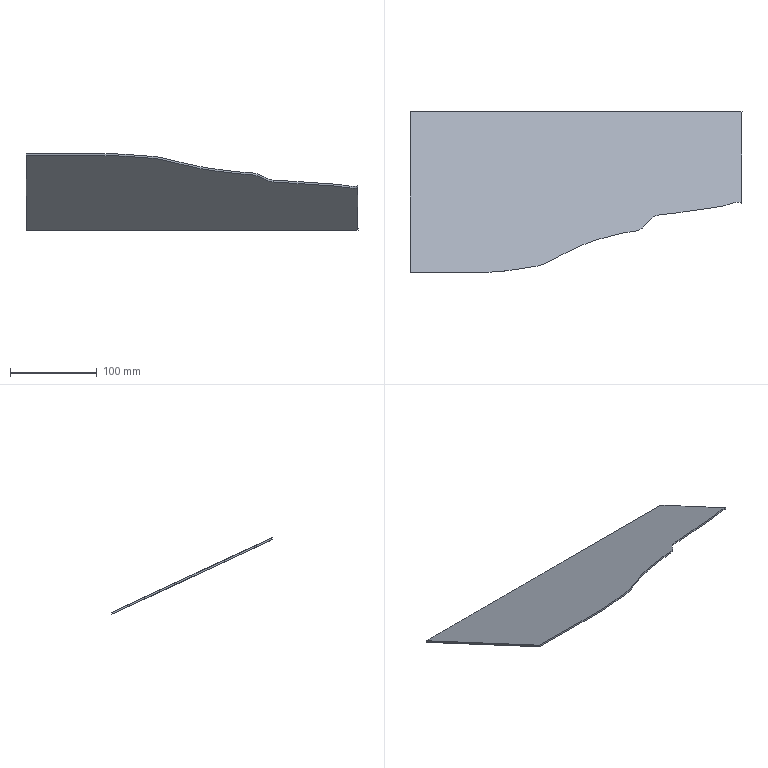Part | NX | features solid 2 | 1 solid | 6 faces | box 382.317 x 185.073 x 88.508 mm | volume 128525 mm3 | plane 5 | spline 1
STEP:
#1=CARTESIAN_POINT('',(772.317,314.401,-112.597));
#2=VERTEX_POINT('',#1);
#3=CARTESIAN_POINT('',(772.317,314.401,-110.39));
#4=VERTEX_POINT('',#3);
#5=CARTESIAN_POINT('',(772.317,314.401,-108.11));
#6=DIRECTION('',(0.,0.,-1.));
#7=VECTOR('',#6,1000.);
#8=LINE('',#5,#7);
#9=EDGE_CURVE('',#2,#4,#8,.F.);
#10=ORIENTED_EDGE('',*,*,#9,.F.);
#11=CARTESIAN_POINT('',(772.317,419.993,-161.836));
#12=VERTEX_POINT('',#11);
#13=CARTESIAN_POINT('',(772.317,324.603,-117.355));
#14=DIRECTION('',(0.,-0.9063,0.4226));
#15=VECTOR('',#14,1000.);
#16=LINE('',#13,#15);
#17=EDGE_CURVE('',#12,#2,#16,.T.);
#18=ORIENTED_EDGE('',*,*,#17,.F.);
#19=CARTESIAN_POINT('',(772.317,419.993,-159.629));
#20=VERTEX_POINT('',#19);
#21=CARTESIAN_POINT('',(772.317,419.993,-185.));
#22=DIRECTION('',(0.,0.,1.));
#23=VECTOR('',#22,1000.);
#24=LINE('',#21,#23);
#25=EDGE_CURVE('',#20,#12,#24,.F.);
#26=ORIENTED_EDGE('',*,*,#25,.F.);
#27=CARTESIAN_POINT('',(772.317,325.448,-115.542));
#28=DIRECTION('',(0.,-0.9063,0.4226));
#29=VECTOR('',#28,1000.);
#30=LINE('',#27,#29);
#31=EDGE_CURVE('',#20,#4,#30,.T.);
#32=ORIENTED_EDGE('',*,*,#31,.T.);
#33=EDGE_LOOP('',(#10,#18,#26,#32));
#34=FACE_BOUND('',#33,.T.);
#35=CARTESIAN_POINT('',(772.317,305.865,-157.54));
#36=DIRECTION('',(1.,0.,0.));
#37=DIRECTION('',(0.,1.,0.));
#38=AXIS2_PLACEMENT_3D('',#35,#36,#37);
#39=PLANE('',#38);
#40=ADVANCED_FACE('',(#34),#39,.T.);
#41=CARTESIAN_POINT('',(390.,419.993,-159.629));
#42=VERTEX_POINT('',#41);
#43=CARTESIAN_POINT('',(390.,419.993,-161.836));
#44=VERTEX_POINT('',#43);
#45=CARTESIAN_POINT('',(390.,419.993,-277.54));
#46=DIRECTION('',(0.,0.,-1.));
#47=VECTOR('',#46,1000.);
#48=LINE('',#45,#47);
#49=EDGE_CURVE('',#42,#44,#48,.T.);
#50=ORIENTED_EDGE('',*,*,#49,.F.);
#51=CARTESIAN_POINT('',(750.,419.993,-159.629));
#52=DIRECTION('',(1.,0.,0.));
#53=VECTOR('',#52,1000.);
#54=LINE('',#51,#53);
#55=EDGE_CURVE('',#20,#42,#54,.F.);
#56=ORIENTED_EDGE('',*,*,#55,.F.);
#57=ORIENTED_EDGE('',*,*,#25,.T.);
#58=CARTESIAN_POINT('',(750.,419.993,-161.836));
#59=DIRECTION('',(1.,0.,0.));
#60=VECTOR('',#59,1000.);
#61=LINE('',#58,#60);
#62=EDGE_CURVE('',#12,#44,#61,.F.);
#63=ORIENTED_EDGE('',*,*,#62,.T.);
#64=EDGE_LOOP('',(#50,#56,#57,#63));
#65=FACE_BOUND('',#64,.T.);
#66=CARTESIAN_POINT('',(747.317,419.993,-185.));
#67=DIRECTION('',(0.,-1.,0.));
#68=DIRECTION('',(1.,0.,0.));
#69=AXIS2_PLACEMENT_3D('',#66,#67,#68);
#70=PLANE('',#69);
#71=ADVANCED_FACE('',(#65),#70,.F.);
#72=ORIENTED_EDGE('',*,*,#17,.T.);
#73=CARTESIAN_POINT('',(390.,234.962,-75.554));
#74=VERTEX_POINT('',#73);
#75=CARTESIAN_POINT('',(772.317,314.401,-112.597));
#76=CARTESIAN_POINT('',(771.447,314.942,-112.85));
#77=CARTESIAN_POINT('',(769.521,315.772,-113.237));
#78=CARTESIAN_POINT('',(766.298,315.92,-113.306));
#79=CARTESIAN_POINT('',(763.2,315.367,-113.048));
#80=CARTESIAN_POINT('',(759.218,314.091,-112.453));
#81=CARTESIAN_POINT('',(754.335,312.121,-111.534));
#82=CARTESIAN_POINT('',(748.252,310.6,-110.825));
#83=CARTESIAN_POINT('',(741.925,309.977,-110.534));
#84=CARTESIAN_POINT('',(735.621,309.287,-110.213));
#85=CARTESIAN_POINT('',(729.381,308.282,-109.744));
#86=CARTESIAN_POINT('',(721.074,306.854,-109.078));
#87=CARTESIAN_POINT('',(712.671,305.963,-108.663));
#88=CARTESIAN_POINT('',(704.342,304.659,-108.054));
#89=CARTESIAN_POINT('',(698.124,303.522,-107.524));
#90=CARTESIAN_POINT('',(691.868,302.596,-107.093));
#91=CARTESIAN_POINT('',(685.555,301.997,-106.813));
#92=CARTESIAN_POINT('',(679.228,301.472,-106.569));
#93=CARTESIAN_POINT('',(674.053,300.433,-106.084));
#94=CARTESIAN_POINT('',(670.193,298.785,-105.315));
#95=CARTESIAN_POINT('',(666.812,296.505,-104.252));
#96=CARTESIAN_POINT('',(663.454,292.769,-102.51));
#97=CARTESIAN_POINT('',(659.951,287.939,-100.258));
#98=CARTESIAN_POINT('',(656.127,284.572,-98.688));
#99=CARTESIAN_POINT('',(652.217,282.974,-97.943));
#100=CARTESIAN_POINT('',(648.116,282.1,-97.535));
#101=CARTESIAN_POINT('',(642.775,281.711,-97.354));
#102=CARTESIAN_POINT('',(636.496,280.796,-96.927));
#103=CARTESIAN_POINT('',(630.409,279.139,-96.154));
#104=CARTESIAN_POINT('',(624.399,277.192,-95.247));
#105=CARTESIAN_POINT('',(618.29,275.625,-94.516));
#106=CARTESIAN_POINT('',(612.092,274.233,-93.867));
#107=CARTESIAN_POINT('',(603.916,272.197,-92.917));
#108=CARTESIAN_POINT('',(594.109,268.78,-91.324));
#109=CARTESIAN_POINT('',(582.726,263.871,-89.035));
#110=CARTESIAN_POINT('',(571.594,258.432,-86.499));
#111=CARTESIAN_POINT('',(562.421,253.692,-84.288));
#112=CARTESIAN_POINT('',(555.177,249.676,-82.416));
#113=CARTESIAN_POINT('',(549.724,246.714,-81.035));
#114=CARTESIAN_POINT('',(544.121,244.165,-79.846));
#115=CARTESIAN_POINT('',(536.273,241.806,-78.746));
#116=CARTESIAN_POINT('',(525.864,240.511,-78.142));
#117=CARTESIAN_POINT('',(513.615,238.27,-77.097));
#118=CARTESIAN_POINT('',(501.283,236.342,-76.198));
#119=CARTESIAN_POINT('',(488.945,235.234,-75.681));
#120=CARTESIAN_POINT('',(476.583,234.912,-75.531));
#121=CARTESIAN_POINT('',(460.089,235.002,-75.573));
#122=CARTESIAN_POINT('',(439.477,234.9,-75.526));
#123=CARTESIAN_POINT('',(414.738,234.935,-75.542));
#124=CARTESIAN_POINT('',(398.246,234.96,-75.554));
#125=CARTESIAN_POINT('',(390.,234.962,-75.554));
#126=B_SPLINE_CURVE_WITH_KNOTS('',3,(#75,#76,#77,#78,#79,#80,#81,#82,#83,#84,#85,#86,#87,#88,#89,#90,#91,#92,#93,#94,#95,#96,#97,#98,#99,#100,#101,#102,#103,#104,#105,#106,#107,#108,#109,#110,#111,#112,#113,#114,#115,#116,#117,#118,#119,#120,#121,#122,#123,#124,#125),.UNSPECIFIED.,.F.,.F.,(4,1,1,1,1,1,1,1,1,1,1,1,1,1,1,1,1,1,1,1,1,1,1,1,1,1,1,1,1,1,1,1,1,1,1,1,1,1,1,1,1,1,1,1,1,1,1,1,4),(0.009575,0.0127,0.01583,0.01896,0.02209,0.02834,0.0346,0.04085,0.04711,0.05337,0.05962,0.07214,0.07839,0.08465,0.0909,0.09716,0.1034,0.1097,0.1128,0.1159,0.1222,0.1284,0.1347,0.1378,0.141,0.1472,0.1535,0.1597,0.166,0.1722,0.1785,0.1847,0.1973,0.2098,0.2223,0.2348,0.241,0.2473,0.2536,0.2598,0.2723,0.2848,0.2974,0.3099,0.3224,0.3349,0.3599,0.3849,0.41),.UNSPECIFIED.);
#127=EDGE_CURVE('',#2,#74,#126,.T.);
#128=ORIENTED_EDGE('',*,*,#127,.T.);
#129=CARTESIAN_POINT('',(390.,587.452,-239.923));
#130=DIRECTION('',(0.,0.9063,-0.4226));
#131=VECTOR('',#130,1000.);
#132=LINE('',#129,#131);
#133=EDGE_CURVE('',#44,#74,#132,.F.);
#134=ORIENTED_EDGE('',*,*,#133,.F.);
#135=ORIENTED_EDGE('',*,*,#62,.F.);
#136=EDGE_LOOP('',(#72,#128,#134,#135));
#137=FACE_BOUND('',#136,.T.);
#138=CARTESIAN_POINT('',(750.,587.452,-239.923));
#139=DIRECTION('',(0.,0.4226,0.9063));
#140=DIRECTION('',(1.,0.,0.));
#141=AXIS2_PLACEMENT_3D('',#138,#139,#140);
#142=PLANE('',#141);
#143=ADVANCED_FACE('',(#137),#142,.F.);
#144=CARTESIAN_POINT('',(390.,234.962,-73.348));
#145=VERTEX_POINT('',#144);
#146=CARTESIAN_POINT('',(390.,234.962,-74.448));
#147=DIRECTION('',(0.,0.,-1.));
#148=VECTOR('',#147,1000.);
#149=LINE('',#146,#148);
#150=EDGE_CURVE('',#145,#74,#149,.T.);
#151=ORIENTED_EDGE('',*,*,#150,.F.);
#152=CARTESIAN_POINT('',(390.,588.297,-238.11));
#153=DIRECTION('',(0.,0.9063,-0.4226));
#154=VECTOR('',#153,1000.);
#155=LINE('',#152,#154);
#156=EDGE_CURVE('',#42,#145,#155,.F.);
#157=ORIENTED_EDGE('',*,*,#156,.F.);
#158=ORIENTED_EDGE('',*,*,#49,.T.);
#159=ORIENTED_EDGE('',*,*,#133,.T.);
#160=EDGE_LOOP('',(#151,#157,#158,#159));
#161=FACE_BOUND('',#160,.T.);
#162=CARTESIAN_POINT('',(390.,229.934,-277.54));
#163=DIRECTION('',(1.,-0.000000001,0.));
#164=DIRECTION('',(0.000000001,1.,0.));
#165=AXIS2_PLACEMENT_3D('',#162,#163,#164);
#166=PLANE('',#165);
#167=ADVANCED_FACE('',(#161),#166,.F.);
#168=CARTESIAN_POINT('',(772.317,314.401,-110.39));
#169=CARTESIAN_POINT('',(771.447,314.942,-110.643));
#170=CARTESIAN_POINT('',(769.521,315.772,-111.03));
#171=CARTESIAN_POINT('',(766.298,315.92,-111.099));
#172=CARTESIAN_POINT('',(763.2,315.367,-110.841));
#173=CARTESIAN_POINT('',(759.218,314.091,-110.246));
#174=CARTESIAN_POINT('',(754.335,312.121,-109.327));
#175=CARTESIAN_POINT('',(748.252,310.6,-108.618));
#176=CARTESIAN_POINT('',(741.925,309.977,-108.328));
#177=CARTESIAN_POINT('',(735.621,309.287,-108.006));
#178=CARTESIAN_POINT('',(729.381,308.282,-107.537));
#179=CARTESIAN_POINT('',(721.074,306.854,-106.871));
#180=CARTESIAN_POINT('',(712.671,305.963,-106.456));
#181=CARTESIAN_POINT('',(704.342,304.659,-105.848));
#182=CARTESIAN_POINT('',(698.124,303.522,-105.318));
#183=CARTESIAN_POINT('',(691.868,302.596,-104.886));
#184=CARTESIAN_POINT('',(685.555,301.997,-104.607));
#185=CARTESIAN_POINT('',(679.228,301.472,-104.362));
#186=CARTESIAN_POINT('',(674.053,300.433,-103.877));
#187=CARTESIAN_POINT('',(670.193,298.785,-103.109));
#188=CARTESIAN_POINT('',(666.812,296.505,-102.046));
#189=CARTESIAN_POINT('',(663.454,292.769,-100.303));
#190=CARTESIAN_POINT('',(659.951,287.939,-98.051));
#191=CARTESIAN_POINT('',(656.127,284.572,-96.481));
#192=CARTESIAN_POINT('',(652.217,282.974,-95.736));
#193=CARTESIAN_POINT('',(648.116,282.1,-95.329));
#194=CARTESIAN_POINT('',(642.775,281.711,-95.147));
#195=CARTESIAN_POINT('',(636.496,280.796,-94.72));
#196=CARTESIAN_POINT('',(630.409,279.139,-93.948));
#197=CARTESIAN_POINT('',(624.399,277.192,-93.04));
#198=CARTESIAN_POINT('',(618.29,275.625,-92.309));
#199=CARTESIAN_POINT('',(612.092,274.233,-91.66));
#200=CARTESIAN_POINT('',(603.916,272.197,-90.711));
#201=CARTESIAN_POINT('',(594.109,268.78,-89.117));
#202=CARTESIAN_POINT('',(582.726,263.871,-86.828));
#203=CARTESIAN_POINT('',(571.594,258.432,-84.292));
#204=CARTESIAN_POINT('',(562.421,253.692,-82.082));
#205=CARTESIAN_POINT('',(555.177,249.676,-80.209));
#206=CARTESIAN_POINT('',(549.724,246.714,-78.828));
#207=CARTESIAN_POINT('',(544.121,244.165,-77.639));
#208=CARTESIAN_POINT('',(536.273,241.806,-76.539));
#209=CARTESIAN_POINT('',(525.864,240.511,-75.935));
#210=CARTESIAN_POINT('',(513.615,238.27,-74.89));
#211=CARTESIAN_POINT('',(501.283,236.342,-73.991));
#212=CARTESIAN_POINT('',(488.945,235.234,-73.475));
#213=CARTESIAN_POINT('',(476.583,234.912,-73.324));
#214=CARTESIAN_POINT('',(460.089,235.002,-73.366));
#215=CARTESIAN_POINT('',(439.477,234.9,-73.319));
#216=CARTESIAN_POINT('',(414.738,234.935,-73.335));
#217=CARTESIAN_POINT('',(398.246,234.96,-73.347));
#218=CARTESIAN_POINT('',(390.,234.962,-73.348));
#219=B_SPLINE_CURVE_WITH_KNOTS('',3,(#168,#169,#170,#171,#172,#173,#174,#175,#176,#177,#178,#179,#180,#181,#182,#183,#184,#185,#186,#187,#188,#189,#190,#191,#192,#193,#194,#195,#196,#197,#198,#199,#200,#201,#202,#203,#204,#205,#206,#207,#208,#209,#210,#211,#212,#213,#214,#215,#216,#217,#218),.UNSPECIFIED.,.F.,.F.,(4,1,1,1,1,1,1,1,1,1,1,1,1,1,1,1,1,1,1,1,1,1,1,1,1,1,1,1,1,1,1,1,1,1,1,1,1,1,1,1,1,1,1,1,1,1,1,1,4),(0.009575,0.0127,0.01583,0.01896,0.02209,0.02834,0.0346,0.04085,0.04711,0.05337,0.05962,0.07214,0.07839,0.08465,0.0909,0.09716,0.1034,0.1097,0.1128,0.1159,0.1222,0.1284,0.1347,0.1378,0.141,0.1472,0.1535,0.1597,0.166,0.1722,0.1785,0.1847,0.1973,0.2098,0.2223,0.2348,0.241,0.2473,0.2536,0.2598,0.2723,0.2848,0.2974,0.3099,0.3224,0.3349,0.3599,0.3849,0.41),.UNSPECIFIED.);
#220=EDGE_CURVE('',#4,#145,#219,.T.);
#221=ORIENTED_EDGE('',*,*,#220,.F.);
#222=ORIENTED_EDGE('',*,*,#31,.F.);
#223=ORIENTED_EDGE('',*,*,#55,.T.);
#224=ORIENTED_EDGE('',*,*,#156,.T.);
#225=EDGE_LOOP('',(#221,#222,#223,#224));
#226=FACE_BOUND('',#225,.T.);
#227=CARTESIAN_POINT('',(750.,588.297,-238.11));
#228=DIRECTION('',(0.,0.4226,0.9063));
#229=DIRECTION('',(1.,0.,0.));
#230=AXIS2_PLACEMENT_3D('',#227,#228,#229);
#231=PLANE('',#230);
#232=ADVANCED_FACE('',(#226),#231,.T.);
#233=ORIENTED_EDGE('',*,*,#9,.T.);
#234=ORIENTED_EDGE('',*,*,#220,.T.);
#235=ORIENTED_EDGE('',*,*,#150,.T.);
#236=ORIENTED_EDGE('',*,*,#127,.F.);
#237=EDGE_LOOP('',(#233,#234,#235,#236));
#238=FACE_BOUND('',#237,.T.);
#239=CARTESIAN_POINT('',(390.,234.962,-71.384));
#240=CARTESIAN_POINT('',(390.,234.962,-113.531));
#241=CARTESIAN_POINT('',(398.312,234.96,-71.384));
#242=CARTESIAN_POINT('',(398.312,234.96,-113.531));
#243=CARTESIAN_POINT('',(414.937,234.935,-71.384));
#244=CARTESIAN_POINT('',(414.937,234.935,-113.531));
#245=CARTESIAN_POINT('',(439.875,234.902,-71.384));
#246=CARTESIAN_POINT('',(439.875,234.902,-113.531));
#247=CARTESIAN_POINT('',(460.655,235.002,-71.384));
#248=CARTESIAN_POINT('',(460.655,235.002,-113.531));
#249=CARTESIAN_POINT('',(477.283,234.91,-71.384));
#250=CARTESIAN_POINT('',(477.283,234.91,-113.531));
#251=CARTESIAN_POINT('',(489.746,235.282,-71.384));
#252=CARTESIAN_POINT('',(489.746,235.282,-113.531));
#253=CARTESIAN_POINT('',(502.173,236.446,-71.384));
#254=CARTESIAN_POINT('',(502.173,236.446,-113.531));
#255=CARTESIAN_POINT('',(514.478,238.442,-71.384));
#256=CARTESIAN_POINT('',(514.478,238.442,-113.531));
#257=CARTESIAN_POINT('',(526.748,240.624,-71.384));
#258=CARTESIAN_POINT('',(526.748,240.624,-113.531));
#259=CARTESIAN_POINT('',(537.124,241.952,-71.384));
#260=CARTESIAN_POINT('',(537.124,241.952,-113.531));
#261=CARTESIAN_POINT('',(544.997,244.513,-71.384));
#262=CARTESIAN_POINT('',(544.997,244.513,-113.531));
#263=CARTESIAN_POINT('',(550.635,247.183,-71.384));
#264=CARTESIAN_POINT('',(550.635,247.183,-113.531));
#265=CARTESIAN_POINT('',(556.112,250.205,-71.384));
#266=CARTESIAN_POINT('',(556.112,250.205,-113.531));
#267=CARTESIAN_POINT('',(563.412,254.214,-71.384));
#268=CARTESIAN_POINT('',(563.412,254.214,-113.531));
#269=CARTESIAN_POINT('',(572.64,258.959,-71.384));
#270=CARTESIAN_POINT('',(572.64,258.959,-113.531));
#271=CARTESIAN_POINT('',(583.861,264.397,-71.384));
#272=CARTESIAN_POINT('',(583.861,264.397,-113.531));
#273=CARTESIAN_POINT('',(595.349,269.271,-71.384));
#274=CARTESIAN_POINT('',(595.349,269.271,-113.531));
#275=CARTESIAN_POINT('',(605.214,272.571,-71.384));
#276=CARTESIAN_POINT('',(605.214,272.571,-113.531));
#277=CARTESIAN_POINT('',(613.3,274.506,-71.384));
#278=CARTESIAN_POINT('',(613.3,274.506,-113.531));
#279=CARTESIAN_POINT('',(619.386,275.877,-71.384));
#280=CARTESIAN_POINT('',(619.386,275.877,-113.531));
#281=CARTESIAN_POINT('',(625.4,277.505,-71.384));
#282=CARTESIAN_POINT('',(625.4,277.505,-113.531));
#283=CARTESIAN_POINT('',(631.334,279.423,-71.384));
#284=CARTESIAN_POINT('',(631.334,279.423,-113.531));
#285=CARTESIAN_POINT('',(637.385,280.981,-71.384));
#286=CARTESIAN_POINT('',(637.385,280.981,-113.531));
#287=CARTESIAN_POINT('',(643.568,281.765,-71.384));
#288=CARTESIAN_POINT('',(643.568,281.765,-113.531));
#289=CARTESIAN_POINT('',(649.786,282.237,-71.384));
#290=CARTESIAN_POINT('',(649.786,282.237,-113.531));
#291=CARTESIAN_POINT('',(655.854,284.158,-71.384));
#292=CARTESIAN_POINT('',(655.854,284.158,-113.531));
#293=CARTESIAN_POINT('',(660.412,288.499,-71.384));
#294=CARTESIAN_POINT('',(660.412,288.499,-113.531));
#295=CARTESIAN_POINT('',(664.057,293.596,-71.384));
#296=CARTESIAN_POINT('',(664.057,293.596,-113.531));
#297=CARTESIAN_POINT('',(668.494,298.094,-71.384));
#298=CARTESIAN_POINT('',(668.494,298.094,-113.531));
#299=CARTESIAN_POINT('',(674.252,300.584,-71.384));
#300=CARTESIAN_POINT('',(674.252,300.584,-113.531));
#301=CARTESIAN_POINT('',(680.468,301.604,-71.384));
#302=CARTESIAN_POINT('',(680.468,301.604,-113.531));
#303=CARTESIAN_POINT('',(686.669,302.08,-71.384));
#304=CARTESIAN_POINT('',(686.669,302.08,-113.531));
#305=CARTESIAN_POINT('',(692.875,302.724,-71.384));
#306=CARTESIAN_POINT('',(692.875,302.724,-113.531));
#307=CARTESIAN_POINT('',(699.034,303.686,-71.384));
#308=CARTESIAN_POINT('',(699.034,303.686,-113.531));
#309=CARTESIAN_POINT('',(705.17,304.8,-71.384));
#310=CARTESIAN_POINT('',(705.17,304.8,-113.531));
#311=CARTESIAN_POINT('',(713.389,306.048,-71.384));
#312=CARTESIAN_POINT('',(713.389,306.048,-113.531));
#313=CARTESIAN_POINT('',(721.657,306.942,-71.384));
#314=CARTESIAN_POINT('',(721.657,306.942,-113.531));
#315=CARTESIAN_POINT('',(729.848,308.363,-71.384));
#316=CARTESIAN_POINT('',(729.848,308.363,-113.531));
#317=CARTESIAN_POINT('',(736.006,309.34,-71.384));
#318=CARTESIAN_POINT('',(736.006,309.34,-113.531));
#319=CARTESIAN_POINT('',(742.208,309.998,-71.384));
#320=CARTESIAN_POINT('',(742.208,309.998,-113.531));
#321=CARTESIAN_POINT('',(748.415,310.63,-71.384));
#322=CARTESIAN_POINT('',(748.415,310.63,-113.531));
#323=CARTESIAN_POINT('',(754.47,312.168,-71.384));
#324=CARTESIAN_POINT('',(754.47,312.168,-113.531));
#325=CARTESIAN_POINT('',(760.268,314.517,-71.384));
#326=CARTESIAN_POINT('',(760.268,314.517,-113.531));
#327=CARTESIAN_POINT('',(765.297,315.968,-71.384));
#328=CARTESIAN_POINT('',(765.297,315.968,-113.531));
#329=CARTESIAN_POINT('',(769.495,315.773,-71.384));
#330=CARTESIAN_POINT('',(769.495,315.773,-113.531));
#331=CARTESIAN_POINT('',(771.435,314.95,-71.384));
#332=CARTESIAN_POINT('',(771.435,314.95,-113.531));
#333=CARTESIAN_POINT('',(772.317,314.401,-71.384));
#334=CARTESIAN_POINT('',(772.317,314.401,-113.531));
#335=B_SPLINE_SURFACE_WITH_KNOTS('',3,1,((#239,#240),(#241,#242),(#243,#244),(#245,#246),(#247,#248),(#249,#250),(#251,#252),(#253,#254),(#255,#256),(#257,#258),(#259,#260),(#261,#262),(#263,#264),(#265,#266),(#267,#268),(#269,#270),(#271,#272),(#273,#274),(#275,#276),(#277,#278),(#279,#280),(#281,#282),(#283,#284),(#285,#286),(#287,#288),(#289,#290),(#291,#292),(#293,#294),(#295,#296),(#297,#298),(#299,#300),(#301,#302),(#303,#304),(#305,#306),(#307,#308),(#309,#310),(#311,#312),(#313,#314),(#315,#316),(#317,#318),(#319,#320),(#321,#322),(#323,#324),(#325,#326),(#327,#328),(#329,#330),(#331,#332),(#333,#334)),.SURF_OF_LINEAR_EXTRUSION.,.F.,.F.,.F.,(4,1,1,1,1,1,1,1,1,1,1,1,1,1,1,1,1,1,1,1,1,1,1,1,1,1,1,1,1,1,1,1,1,1,1,1,1,1,1,1,1,1,1,1,1,4),(2,2),(0.8226,0.8281,0.8336,0.8391,0.8418,0.8446,0.8473,0.8501,0.8528,0.8555,0.8569,0.8583,0.8597,0.861,0.8638,0.8665,0.8693,0.872,0.8734,0.8747,0.8761,0.8775,0.8788,0.8802,0.8816,0.883,0.8843,0.8857,0.8871,0.8884,0.8898,0.8912,0.8926,0.8939,0.8953,0.8967,0.8994,0.9008,0.9022,0.9035,0.9049,0.9063,0.9076,0.909,0.9097,0.9104),(0.,1.),.UNSPECIFIED.);
#336=ADVANCED_FACE('',(#238),#335,.F.);
#337=CLOSED_SHELL('',(#40,#71,#143,#167,#232,#336));
#338=MANIFOLD_SOLID_BREP('',#337);
#339=(LENGTH_UNIT()NAMED_UNIT(*)SI_UNIT(.MILLI.,.METRE.));
#340=UNCERTAINTY_MEASURE_WITH_UNIT(LENGTH_MEASURE(0.0508),#339,'','');
#341=(NAMED_UNIT(*)PLANE_ANGLE_UNIT()SI_UNIT($,.RADIAN.));
#342=(NAMED_UNIT(*)SI_UNIT($,.STERADIAN.)SOLID_ANGLE_UNIT());
#343=(GEOMETRIC_REPRESENTATION_CONTEXT(3)GLOBAL_UNCERTAINTY_ASSIGNED_CONTEXT((#340))GLOBAL_UNIT_ASSIGNED_CONTEXT((#339,#341,#342))REPRESENTATION_CONTEXT('',''));
#344=ADVANCED_BREP_SHAPE_REPRESENTATION('',(#338),#343);